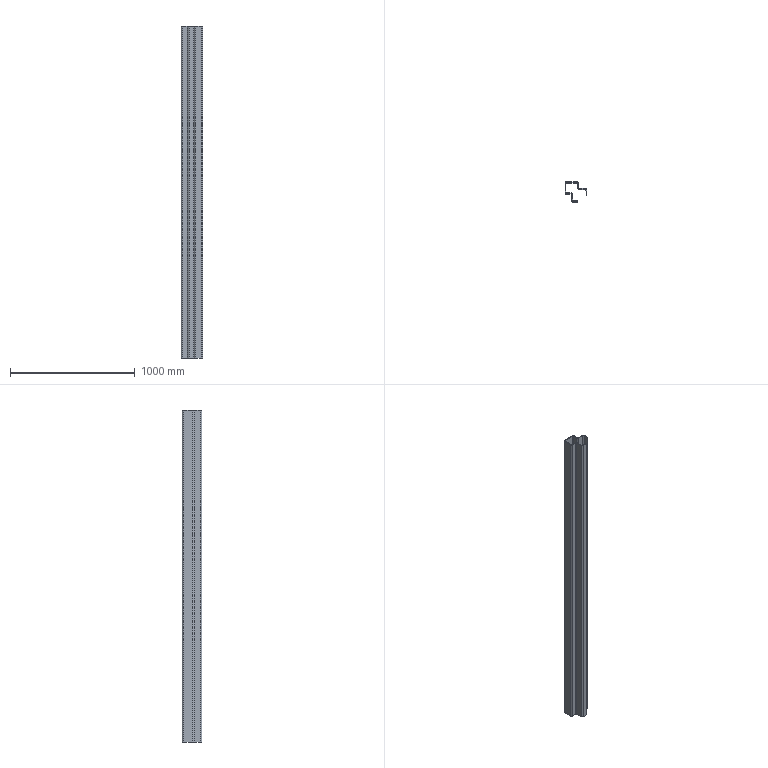Part | SolidWorks | features Extrusion 1 | 1 solid | 34 faces | box 174 x 158 x 2660 mm | volume 7867644 mm3 | plane 20 | cylinder 14 | commonest cylinder face diameters 12 x7 24 x7
STEP:
#1=CARTESIAN_POINT('',(-6.,0.,0.));
#2=VERTEX_POINT('',#1);
#3=CARTESIAN_POINT('',(0.,0.,0.));
#4=VERTEX_POINT('',#3);
#5=CARTESIAN_POINT('',(-6.,0.,0.));
#6=DIRECTION('',(1.,0.,0.));
#7=VECTOR('',#6,1000.);
#8=LINE('',#5,#7);
#9=EDGE_CURVE('',#2,#4,#8,.T.);
#10=ORIENTED_EDGE('',*,*,#9,.T.);
#11=CARTESIAN_POINT('',(0.,0.,2660.));
#12=VERTEX_POINT('',#11);
#13=CARTESIAN_POINT('',(0.,0.,2660.));
#14=DIRECTION('',(0.,0.,-1.));
#15=VECTOR('',#14,1000.);
#16=LINE('',#13,#15);
#17=EDGE_CURVE('',#12,#4,#16,.T.);
#18=ORIENTED_EDGE('',*,*,#17,.F.);
#19=CARTESIAN_POINT('',(-6.,0.,2660.));
#20=VERTEX_POINT('',#19);
#21=CARTESIAN_POINT('',(-6.,0.,2660.));
#22=DIRECTION('',(1.,0.,0.));
#23=VECTOR('',#22,1000.);
#24=LINE('',#21,#23);
#25=EDGE_CURVE('',#20,#12,#24,.T.);
#26=ORIENTED_EDGE('',*,*,#25,.F.);
#27=CARTESIAN_POINT('',(-6.,0.,2660.));
#28=DIRECTION('',(0.,0.,-1.));
#29=VECTOR('',#28,1000.);
#30=LINE('',#27,#29);
#31=EDGE_CURVE('',#20,#2,#30,.T.);
#32=ORIENTED_EDGE('',*,*,#31,.T.);
#33=EDGE_LOOP('',(#10,#18,#26,#32));
#34=FACE_OUTER_BOUND('',#33,.T.);
#35=CARTESIAN_POINT('',(-6.,0.,2660.));
#36=DIRECTION('',(0.,1.,0.));
#37=DIRECTION('',(0.,0.,1.));
#38=AXIS2_PLACEMENT_3D('',#35,#36,#37);
#39=PLANE('',#38);
#40=ADVANCED_FACE('',(#34),#39,.F.);
#41=CARTESIAN_POINT('',(0.,38.,0.));
#42=VERTEX_POINT('',#41);
#43=CARTESIAN_POINT('',(0.,0.,0.));
#44=DIRECTION('',(0.,1.,0.));
#45=VECTOR('',#44,1000.);
#46=LINE('',#43,#45);
#47=EDGE_CURVE('',#4,#42,#46,.T.);
#48=ORIENTED_EDGE('',*,*,#47,.T.);
#49=CARTESIAN_POINT('',(0.,38.,2660.));
#50=VERTEX_POINT('',#49);
#51=CARTESIAN_POINT('',(0.,38.,2660.));
#52=DIRECTION('',(0.,0.,-1.));
#53=VECTOR('',#52,1000.);
#54=LINE('',#51,#53);
#55=EDGE_CURVE('',#50,#42,#54,.T.);
#56=ORIENTED_EDGE('',*,*,#55,.F.);
#57=CARTESIAN_POINT('',(0.,0.,2660.));
#58=DIRECTION('',(0.,1.,0.));
#59=VECTOR('',#58,1000.);
#60=LINE('',#57,#59);
#61=EDGE_CURVE('',#12,#50,#60,.T.);
#62=ORIENTED_EDGE('',*,*,#61,.F.);
#63=ORIENTED_EDGE('',*,*,#17,.T.);
#64=EDGE_LOOP('',(#48,#56,#62,#63));
#65=FACE_OUTER_BOUND('',#64,.T.);
#66=CARTESIAN_POINT('',(0.,0.,2660.));
#67=DIRECTION('',(-1.,0.,0.));
#68=DIRECTION('',(0.,0.,1.));
#69=AXIS2_PLACEMENT_3D('',#66,#67,#68);
#70=PLANE('',#69);
#71=ADVANCED_FACE('',(#65),#70,.F.);
#72=CARTESIAN_POINT('',(-12.,50.,0.));
#73=VERTEX_POINT('',#72);
#74=CARTESIAN_POINT('',(-12.,38.,0.));
#75=DIRECTION('',(0.,0.,1.));
#76=DIRECTION('',(1.,0.,0.));
#77=AXIS2_PLACEMENT_3D('',#74,#75,#76);
#78=CIRCLE('',#77,12.);
#79=EDGE_CURVE('',#42,#73,#78,.T.);
#80=ORIENTED_EDGE('',*,*,#79,.T.);
#81=CARTESIAN_POINT('',(-12.,50.,2660.));
#82=VERTEX_POINT('',#81);
#83=CARTESIAN_POINT('',(-12.,50.,2660.));
#84=DIRECTION('',(0.,0.,-1.));
#85=VECTOR('',#84,1000.);
#86=LINE('',#83,#85);
#87=EDGE_CURVE('',#82,#73,#86,.T.);
#88=ORIENTED_EDGE('',*,*,#87,.F.);
#89=CARTESIAN_POINT('',(-12.,38.,2660.));
#90=DIRECTION('',(0.,0.,1.));
#91=DIRECTION('',(1.,0.,0.));
#92=AXIS2_PLACEMENT_3D('',#89,#90,#91);
#93=CIRCLE('',#92,12.);
#94=EDGE_CURVE('',#50,#82,#93,.T.);
#95=ORIENTED_EDGE('',*,*,#94,.F.);
#96=ORIENTED_EDGE('',*,*,#55,.T.);
#97=EDGE_LOOP('',(#80,#88,#95,#96));
#98=FACE_OUTER_BOUND('',#97,.T.);
#99=CARTESIAN_POINT('',(-12.,38.,2660.));
#100=DIRECTION('',(0.,0.,-1.));
#101=DIRECTION('',(-1.,0.,0.));
#102=AXIS2_PLACEMENT_3D('',#99,#100,#101);
#103=CYLINDRICAL_SURFACE('',#102,12.);
#104=ADVANCED_FACE('',(#98),#103,.T.);
#105=CARTESIAN_POINT('',(-59.,50.,0.));
#106=VERTEX_POINT('',#105);
#107=CARTESIAN_POINT('',(-12.,50.,0.));
#108=DIRECTION('',(-1.,0.,0.));
#109=VECTOR('',#108,1000.);
#110=LINE('',#107,#109);
#111=EDGE_CURVE('',#73,#106,#110,.T.);
#112=ORIENTED_EDGE('',*,*,#111,.T.);
#113=CARTESIAN_POINT('',(-59.,50.,2660.));
#114=VERTEX_POINT('',#113);
#115=CARTESIAN_POINT('',(-59.,50.,2660.));
#116=DIRECTION('',(0.,0.,-1.));
#117=VECTOR('',#116,1000.);
#118=LINE('',#115,#117);
#119=EDGE_CURVE('',#114,#106,#118,.T.);
#120=ORIENTED_EDGE('',*,*,#119,.F.);
#121=CARTESIAN_POINT('',(-12.,50.,2660.));
#122=DIRECTION('',(-1.,0.,0.));
#123=VECTOR('',#122,1000.);
#124=LINE('',#121,#123);
#125=EDGE_CURVE('',#82,#114,#124,.T.);
#126=ORIENTED_EDGE('',*,*,#125,.F.);
#127=ORIENTED_EDGE('',*,*,#87,.T.);
#128=EDGE_LOOP('',(#112,#120,#126,#127));
#129=FACE_OUTER_BOUND('',#128,.T.);
#130=CARTESIAN_POINT('',(-12.,50.,2660.));
#131=DIRECTION('',(0.,-1.,0.));
#132=DIRECTION('',(1.,0.,0.));
#133=AXIS2_PLACEMENT_3D('',#130,#131,#132);
#134=PLANE('',#133);
#135=ADVANCED_FACE('',(#129),#134,.F.);
#136=CARTESIAN_POINT('',(-65.,56.,0.));
#137=VERTEX_POINT('',#136);
#138=CARTESIAN_POINT('',(-59.,56.,0.));
#139=DIRECTION('',(0.,0.,-1.));
#140=DIRECTION('',(1.,0.,0.));
#141=AXIS2_PLACEMENT_3D('',#138,#139,#140);
#142=CIRCLE('',#141,6.);
#143=EDGE_CURVE('',#106,#137,#142,.T.);
#144=ORIENTED_EDGE('',*,*,#143,.T.);
#145=CARTESIAN_POINT('',(-65.,56.,2660.));
#146=VERTEX_POINT('',#145);
#147=CARTESIAN_POINT('',(-65.,56.,2660.));
#148=DIRECTION('',(0.,0.,-1.));
#149=VECTOR('',#148,1000.);
#150=LINE('',#147,#149);
#151=EDGE_CURVE('',#146,#137,#150,.T.);
#152=ORIENTED_EDGE('',*,*,#151,.F.);
#153=CARTESIAN_POINT('',(-59.,56.,2660.));
#154=DIRECTION('',(0.,0.,-1.));
#155=DIRECTION('',(1.,0.,0.));
#156=AXIS2_PLACEMENT_3D('',#153,#154,#155);
#157=CIRCLE('',#156,6.);
#158=EDGE_CURVE('',#114,#146,#157,.T.);
#159=ORIENTED_EDGE('',*,*,#158,.F.);
#160=ORIENTED_EDGE('',*,*,#119,.T.);
#161=EDGE_LOOP('',(#144,#152,#159,#160));
#162=FACE_OUTER_BOUND('',#161,.T.);
#163=CARTESIAN_POINT('',(-59.,56.,2660.));
#164=DIRECTION('',(0.,0.,-1.));
#165=DIRECTION('',(-1.,0.,0.));
#166=AXIS2_PLACEMENT_3D('',#163,#164,#165);
#167=CYLINDRICAL_SURFACE('',#166,6.);
#168=ADVANCED_FACE('',(#162),#167,.F.);
#169=CARTESIAN_POINT('',(-65.,91.,0.));
#170=VERTEX_POINT('',#169);
#171=CARTESIAN_POINT('',(-65.,56.,0.));
#172=DIRECTION('',(0.,1.,0.));
#173=VECTOR('',#172,1000.);
#174=LINE('',#171,#173);
#175=EDGE_CURVE('',#137,#170,#174,.T.);
#176=ORIENTED_EDGE('',*,*,#175,.T.);
#177=CARTESIAN_POINT('',(-65.,91.,2660.));
#178=VERTEX_POINT('',#177);
#179=CARTESIAN_POINT('',(-65.,91.,2660.));
#180=DIRECTION('',(0.,0.,-1.));
#181=VECTOR('',#180,1000.);
#182=LINE('',#179,#181);
#183=EDGE_CURVE('',#178,#170,#182,.T.);
#184=ORIENTED_EDGE('',*,*,#183,.F.);
#185=CARTESIAN_POINT('',(-65.,56.,2660.));
#186=DIRECTION('',(0.,1.,0.));
#187=VECTOR('',#186,1000.);
#188=LINE('',#185,#187);
#189=EDGE_CURVE('',#146,#178,#188,.T.);
#190=ORIENTED_EDGE('',*,*,#189,.F.);
#191=ORIENTED_EDGE('',*,*,#151,.T.);
#192=EDGE_LOOP('',(#176,#184,#190,#191));
#193=FACE_OUTER_BOUND('',#192,.T.);
#194=CARTESIAN_POINT('',(-65.,56.,2660.));
#195=DIRECTION('',(-1.,0.,0.));
#196=DIRECTION('',(0.,-1.,0.));
#197=AXIS2_PLACEMENT_3D('',#194,#195,#196);
#198=PLANE('',#197);
#199=ADVANCED_FACE('',(#193),#198,.F.);
#200=CARTESIAN_POINT('',(-77.,103.,0.));
#201=VERTEX_POINT('',#200);
#202=CARTESIAN_POINT('',(-77.,91.,0.));
#203=DIRECTION('',(0.,0.,1.));
#204=DIRECTION('',(1.,0.,0.));
#205=AXIS2_PLACEMENT_3D('',#202,#203,#204);
#206=CIRCLE('',#205,12.);
#207=EDGE_CURVE('',#170,#201,#206,.T.);
#208=ORIENTED_EDGE('',*,*,#207,.T.);
#209=CARTESIAN_POINT('',(-77.,103.,2660.));
#210=VERTEX_POINT('',#209);
#211=CARTESIAN_POINT('',(-77.,103.,2660.));
#212=DIRECTION('',(0.,0.,-1.));
#213=VECTOR('',#212,1000.);
#214=LINE('',#211,#213);
#215=EDGE_CURVE('',#210,#201,#214,.T.);
#216=ORIENTED_EDGE('',*,*,#215,.F.);
#217=CARTESIAN_POINT('',(-77.,91.,2660.));
#218=DIRECTION('',(0.,0.,1.));
#219=DIRECTION('',(1.,0.,0.));
#220=AXIS2_PLACEMENT_3D('',#217,#218,#219);
#221=CIRCLE('',#220,12.);
#222=EDGE_CURVE('',#178,#210,#221,.T.);
#223=ORIENTED_EDGE('',*,*,#222,.F.);
#224=ORIENTED_EDGE('',*,*,#183,.T.);
#225=EDGE_LOOP('',(#208,#216,#223,#224));
#226=FACE_OUTER_BOUND('',#225,.T.);
#227=CARTESIAN_POINT('',(-77.,91.,2660.));
#228=DIRECTION('',(0.,0.,-1.));
#229=DIRECTION('',(-1.,0.,0.));
#230=AXIS2_PLACEMENT_3D('',#227,#228,#229);
#231=CYLINDRICAL_SURFACE('',#230,12.);
#232=ADVANCED_FACE('',(#226),#231,.T.);
#233=CARTESIAN_POINT('',(-162.,103.,0.));
#234=VERTEX_POINT('',#233);
#235=CARTESIAN_POINT('',(-77.,103.,0.));
#236=DIRECTION('',(-1.,0.,0.));
#237=VECTOR('',#236,1000.);
#238=LINE('',#235,#237);
#239=EDGE_CURVE('',#201,#234,#238,.T.);
#240=ORIENTED_EDGE('',*,*,#239,.T.);
#241=CARTESIAN_POINT('',(-162.,103.,2660.));
#242=VERTEX_POINT('',#241);
#243=CARTESIAN_POINT('',(-162.,103.,2660.));
#244=DIRECTION('',(0.,0.,-1.));
#245=VECTOR('',#244,1000.);
#246=LINE('',#243,#245);
#247=EDGE_CURVE('',#242,#234,#246,.T.);
#248=ORIENTED_EDGE('',*,*,#247,.F.);
#249=CARTESIAN_POINT('',(-77.,103.,2660.));
#250=DIRECTION('',(-1.,0.,0.));
#251=VECTOR('',#250,1000.);
#252=LINE('',#249,#251);
#253=EDGE_CURVE('',#210,#242,#252,.T.);
#254=ORIENTED_EDGE('',*,*,#253,.F.);
#255=ORIENTED_EDGE('',*,*,#215,.T.);
#256=EDGE_LOOP('',(#240,#248,#254,#255));
#257=FACE_OUTER_BOUND('',#256,.T.);
#258=CARTESIAN_POINT('',(-77.,103.,2660.));
#259=DIRECTION('',(0.,-1.,0.));
#260=DIRECTION('',(1.,0.,0.));
#261=AXIS2_PLACEMENT_3D('',#258,#259,#260);
#262=PLANE('',#261);
#263=ADVANCED_FACE('',(#257),#262,.F.);
#264=CARTESIAN_POINT('',(-174.,91.,0.));
#265=VERTEX_POINT('',#264);
#266=CARTESIAN_POINT('',(-162.,91.,0.));
#267=DIRECTION('',(0.,0.,1.));
#268=DIRECTION('',(1.,0.,0.));
#269=AXIS2_PLACEMENT_3D('',#266,#267,#268);
#270=CIRCLE('',#269,12.);
#271=EDGE_CURVE('',#234,#265,#270,.T.);
#272=ORIENTED_EDGE('',*,*,#271,.T.);
#273=CARTESIAN_POINT('',(-174.,91.,2660.));
#274=VERTEX_POINT('',#273);
#275=CARTESIAN_POINT('',(-174.,91.,2660.));
#276=DIRECTION('',(0.,0.,-1.));
#277=VECTOR('',#276,1000.);
#278=LINE('',#275,#277);
#279=EDGE_CURVE('',#274,#265,#278,.T.);
#280=ORIENTED_EDGE('',*,*,#279,.F.);
#281=CARTESIAN_POINT('',(-162.,91.,2660.));
#282=DIRECTION('',(0.,0.,1.));
#283=DIRECTION('',(1.,0.,0.));
#284=AXIS2_PLACEMENT_3D('',#281,#282,#283);
#285=CIRCLE('',#284,12.);
#286=EDGE_CURVE('',#242,#274,#285,.T.);
#287=ORIENTED_EDGE('',*,*,#286,.F.);
#288=ORIENTED_EDGE('',*,*,#247,.T.);
#289=EDGE_LOOP('',(#272,#280,#287,#288));
#290=FACE_OUTER_BOUND('',#289,.T.);
#291=CARTESIAN_POINT('',(-162.,91.,2660.));
#292=DIRECTION('',(0.,0.,-1.));
#293=DIRECTION('',(-1.,0.,0.));
#294=AXIS2_PLACEMENT_3D('',#291,#292,#293);
#295=CYLINDRICAL_SURFACE('',#294,12.);
#296=ADVANCED_FACE('',(#290),#295,.T.);
#297=CARTESIAN_POINT('',(-174.,21.,0.));
#298=VERTEX_POINT('',#297);
#299=CARTESIAN_POINT('',(-174.,91.,0.));
#300=DIRECTION('',(0.,-1.,0.));
#301=VECTOR('',#300,1000.);
#302=LINE('',#299,#301);
#303=EDGE_CURVE('',#265,#298,#302,.T.);
#304=ORIENTED_EDGE('',*,*,#303,.T.);
#305=CARTESIAN_POINT('',(-174.,21.,2660.));
#306=VERTEX_POINT('',#305);
#307=CARTESIAN_POINT('',(-174.,21.,2660.));
#308=DIRECTION('',(0.,0.,-1.));
#309=VECTOR('',#308,1000.);
#310=LINE('',#307,#309);
#311=EDGE_CURVE('',#306,#298,#310,.T.);
#312=ORIENTED_EDGE('',*,*,#311,.F.);
#313=CARTESIAN_POINT('',(-174.,91.,2660.));
#314=DIRECTION('',(0.,-1.,0.));
#315=VECTOR('',#314,1000.);
#316=LINE('',#313,#315);
#317=EDGE_CURVE('',#274,#306,#316,.T.);
#318=ORIENTED_EDGE('',*,*,#317,.F.);
#319=ORIENTED_EDGE('',*,*,#279,.T.);
#320=EDGE_LOOP('',(#304,#312,#318,#319));
#321=FACE_OUTER_BOUND('',#320,.T.);
#322=CARTESIAN_POINT('',(-174.,91.,2660.));
#323=DIRECTION('',(1.,0.,0.));
#324=DIRECTION('',(0.,1.,0.));
#325=AXIS2_PLACEMENT_3D('',#322,#323,#324);
#326=PLANE('',#325);
#327=ADVANCED_FACE('',(#321),#326,.F.);
#328=CARTESIAN_POINT('',(-162.,9.,0.));
#329=VERTEX_POINT('',#328);
#330=CARTESIAN_POINT('',(-162.,21.,0.));
#331=DIRECTION('',(0.,0.,1.));
#332=DIRECTION('',(1.,0.,0.));
#333=AXIS2_PLACEMENT_3D('',#330,#331,#332);
#334=CIRCLE('',#333,12.);
#335=EDGE_CURVE('',#298,#329,#334,.T.);
#336=ORIENTED_EDGE('',*,*,#335,.T.);
#337=CARTESIAN_POINT('',(-162.,9.,2660.));
#338=VERTEX_POINT('',#337);
#339=CARTESIAN_POINT('',(-162.,9.,2660.));
#340=DIRECTION('',(0.,0.,-1.));
#341=VECTOR('',#340,1000.);
#342=LINE('',#339,#341);
#343=EDGE_CURVE('',#338,#329,#342,.T.);
#344=ORIENTED_EDGE('',*,*,#343,.F.);
#345=CARTESIAN_POINT('',(-162.,21.,2660.));
#346=DIRECTION('',(0.,0.,1.));
#347=DIRECTION('',(1.,0.,0.));
#348=AXIS2_PLACEMENT_3D('',#345,#346,#347);
#349=CIRCLE('',#348,12.);
#350=EDGE_CURVE('',#306,#338,#349,.T.);
#351=ORIENTED_EDGE('',*,*,#350,.F.);
#352=ORIENTED_EDGE('',*,*,#311,.T.);
#353=EDGE_LOOP('',(#336,#344,#351,#352));
#354=FACE_OUTER_BOUND('',#353,.T.);
#355=CARTESIAN_POINT('',(-162.,21.,2660.));
#356=DIRECTION('',(0.,0.,-1.));
#357=DIRECTION('',(-1.,0.,0.));
#358=AXIS2_PLACEMENT_3D('',#355,#356,#357);
#359=CYLINDRICAL_SURFACE('',#358,12.);
#360=ADVANCED_FACE('',(#354),#359,.T.);
#361=CARTESIAN_POINT('',(-127.,9.,0.));
#362=VERTEX_POINT('',#361);
#363=CARTESIAN_POINT('',(-162.,9.,0.));
#364=DIRECTION('',(1.,0.,0.));
#365=VECTOR('',#364,1000.);
#366=LINE('',#363,#365);
#367=EDGE_CURVE('',#329,#362,#366,.T.);
#368=ORIENTED_EDGE('',*,*,#367,.T.);
#369=CARTESIAN_POINT('',(-127.,9.,2660.));
#370=VERTEX_POINT('',#369);
#371=CARTESIAN_POINT('',(-127.,9.,2660.));
#372=DIRECTION('',(0.,0.,-1.));
#373=VECTOR('',#372,1000.);
#374=LINE('',#371,#373);
#375=EDGE_CURVE('',#370,#362,#374,.T.);
#376=ORIENTED_EDGE('',*,*,#375,.F.);
#377=CARTESIAN_POINT('',(-162.,9.,2660.));
#378=DIRECTION('',(1.,0.,0.));
#379=VECTOR('',#378,1000.);
#380=LINE('',#377,#379);
#381=EDGE_CURVE('',#338,#370,#380,.T.);
#382=ORIENTED_EDGE('',*,*,#381,.F.);
#383=ORIENTED_EDGE('',*,*,#343,.T.);
#384=EDGE_LOOP('',(#368,#376,#382,#383));
#385=FACE_OUTER_BOUND('',#384,.T.);
#386=CARTESIAN_POINT('',(-162.,9.,2660.));
#387=DIRECTION('',(0.,1.,0.));
#388=DIRECTION('',(0.,0.,1.));
#389=AXIS2_PLACEMENT_3D('',#386,#387,#388);
#390=PLANE('',#389);
#391=ADVANCED_FACE('',(#385),#390,.F.);
#392=CARTESIAN_POINT('',(-121.,3.,0.));
#393=VERTEX_POINT('',#392);
#394=CARTESIAN_POINT('',(-127.,3.,0.));
#395=DIRECTION('',(0.,0.,-1.));
#396=DIRECTION('',(1.,0.,0.));
#397=AXIS2_PLACEMENT_3D('',#394,#395,#396);
#398=CIRCLE('',#397,6.);
#399=EDGE_CURVE('',#362,#393,#398,.T.);
#400=ORIENTED_EDGE('',*,*,#399,.T.);
#401=CARTESIAN_POINT('',(-121.,3.,2660.));
#402=VERTEX_POINT('',#401);
#403=CARTESIAN_POINT('',(-121.,3.,2660.));
#404=DIRECTION('',(0.,0.,-1.));
#405=VECTOR('',#404,1000.);
#406=LINE('',#403,#405);
#407=EDGE_CURVE('',#402,#393,#406,.T.);
#408=ORIENTED_EDGE('',*,*,#407,.F.);
#409=CARTESIAN_POINT('',(-127.,3.,2660.));
#410=DIRECTION('',(0.,0.,-1.));
#411=DIRECTION('',(1.,0.,0.));
#412=AXIS2_PLACEMENT_3D('',#409,#410,#411);
#413=CIRCLE('',#412,6.);
#414=EDGE_CURVE('',#370,#402,#413,.T.);
#415=ORIENTED_EDGE('',*,*,#414,.F.);
#416=ORIENTED_EDGE('',*,*,#375,.T.);
#417=EDGE_LOOP('',(#400,#408,#415,#416));
#418=FACE_OUTER_BOUND('',#417,.T.);
#419=CARTESIAN_POINT('',(-127.,3.,2660.));
#420=DIRECTION('',(0.,0.,-1.));
#421=DIRECTION('',(-1.,0.,0.));
#422=AXIS2_PLACEMENT_3D('',#419,#420,#421);
#423=CYLINDRICAL_SURFACE('',#422,6.);
#424=ADVANCED_FACE('',(#418),#423,.F.);
#425=CARTESIAN_POINT('',(-121.,-43.,0.));
#426=VERTEX_POINT('',#425);
#427=CARTESIAN_POINT('',(-121.,3.,0.));
#428=DIRECTION('',(0.,-1.,0.));
#429=VECTOR('',#428,1000.);
#430=LINE('',#427,#429);
#431=EDGE_CURVE('',#393,#426,#430,.T.);
#432=ORIENTED_EDGE('',*,*,#431,.T.);
#433=CARTESIAN_POINT('',(-121.,-43.,2660.));
#434=VERTEX_POINT('',#433);
#435=CARTESIAN_POINT('',(-121.,-43.,2660.));
#436=DIRECTION('',(0.,0.,-1.));
#437=VECTOR('',#436,1000.);
#438=LINE('',#435,#437);
#439=EDGE_CURVE('',#434,#426,#438,.T.);
#440=ORIENTED_EDGE('',*,*,#439,.F.);
#441=CARTESIAN_POINT('',(-121.,3.,2660.));
#442=DIRECTION('',(0.,-1.,0.));
#443=VECTOR('',#442,1000.);
#444=LINE('',#441,#443);
#445=EDGE_CURVE('',#402,#434,#444,.T.);
#446=ORIENTED_EDGE('',*,*,#445,.F.);
#447=ORIENTED_EDGE('',*,*,#407,.T.);
#448=EDGE_LOOP('',(#432,#440,#446,#447));
#449=FACE_OUTER_BOUND('',#448,.T.);
#450=CARTESIAN_POINT('',(-121.,3.,2660.));
#451=DIRECTION('',(1.,0.,0.));
#452=DIRECTION('',(0.,0.,-1.));
#453=AXIS2_PLACEMENT_3D('',#450,#451,#452);
#454=PLANE('',#453);
#455=ADVANCED_FACE('',(#449),#454,.F.);
#456=CARTESIAN_POINT('',(-109.,-55.,0.));
#457=VERTEX_POINT('',#456);
#458=CARTESIAN_POINT('',(-109.,-43.,0.));
#459=DIRECTION('',(0.,0.,1.));
#460=DIRECTION('',(1.,0.,0.));
#461=AXIS2_PLACEMENT_3D('',#458,#459,#460);
#462=CIRCLE('',#461,12.);
#463=EDGE_CURVE('',#426,#457,#462,.T.);
#464=ORIENTED_EDGE('',*,*,#463,.T.);
#465=CARTESIAN_POINT('',(-109.,-55.,2660.));
#466=VERTEX_POINT('',#465);
#467=CARTESIAN_POINT('',(-109.,-55.,2660.));
#468=DIRECTION('',(0.,0.,-1.));
#469=VECTOR('',#468,1000.);
#470=LINE('',#467,#469);
#471=EDGE_CURVE('',#466,#457,#470,.T.);
#472=ORIENTED_EDGE('',*,*,#471,.F.);
#473=CARTESIAN_POINT('',(-109.,-43.,2660.));
#474=DIRECTION('',(0.,0.,1.));
#475=DIRECTION('',(1.,0.,0.));
#476=AXIS2_PLACEMENT_3D('',#473,#474,#475);
#477=CIRCLE('',#476,12.);
#478=EDGE_CURVE('',#434,#466,#477,.T.);
#479=ORIENTED_EDGE('',*,*,#478,.F.);
#480=ORIENTED_EDGE('',*,*,#439,.T.);
#481=EDGE_LOOP('',(#464,#472,#479,#480));
#482=FACE_OUTER_BOUND('',#481,.T.);
#483=CARTESIAN_POINT('',(-109.,-43.,2660.));
#484=DIRECTION('',(0.,0.,-1.));
#485=DIRECTION('',(-1.,0.,0.));
#486=AXIS2_PLACEMENT_3D('',#483,#484,#485);
#487=CYLINDRICAL_SURFACE('',#486,12.);
#488=ADVANCED_FACE('',(#482),#487,.T.);
#489=CARTESIAN_POINT('',(-71.,-55.,0.));
#490=VERTEX_POINT('',#489);
#491=CARTESIAN_POINT('',(-109.,-55.,0.));
#492=DIRECTION('',(1.,0.,0.));
#493=VECTOR('',#492,1000.);
#494=LINE('',#491,#493);
#495=EDGE_CURVE('',#457,#490,#494,.T.);
#496=ORIENTED_EDGE('',*,*,#495,.T.);
#497=CARTESIAN_POINT('',(-71.,-55.,2660.));
#498=VERTEX_POINT('',#497);
#499=CARTESIAN_POINT('',(-71.,-55.,2660.));
#500=DIRECTION('',(0.,0.,-1.));
#501=VECTOR('',#500,1000.);
#502=LINE('',#499,#501);
#503=EDGE_CURVE('',#498,#490,#502,.T.);
#504=ORIENTED_EDGE('',*,*,#503,.F.);
#505=CARTESIAN_POINT('',(-109.,-55.,2660.));
#506=DIRECTION('',(1.,0.,0.));
#507=VECTOR('',#506,1000.);
#508=LINE('',#505,#507);
#509=EDGE_CURVE('',#466,#498,#508,.T.);
#510=ORIENTED_EDGE('',*,*,#509,.F.);
#511=ORIENTED_EDGE('',*,*,#471,.T.);
#512=EDGE_LOOP('',(#496,#504,#510,#511));
#513=FACE_OUTER_BOUND('',#512,.T.);
#514=CARTESIAN_POINT('',(-109.,-55.,2660.));
#515=DIRECTION('',(0.,1.,0.));
#516=DIRECTION('',(0.,0.,1.));
#517=AXIS2_PLACEMENT_3D('',#514,#515,#516);
#518=PLANE('',#517);
#519=ADVANCED_FACE('',(#513),#518,.F.);
#520=CARTESIAN_POINT('',(-71.,-49.,0.));
#521=VERTEX_POINT('',#520);
#522=CARTESIAN_POINT('',(-71.,-55.,0.));
#523=DIRECTION('',(0.,1.,0.));
#524=VECTOR('',#523,1000.);
#525=LINE('',#522,#524);
#526=EDGE_CURVE('',#490,#521,#525,.T.);
#527=ORIENTED_EDGE('',*,*,#526,.T.);
#528=CARTESIAN_POINT('',(-71.,-49.,2660.));
#529=VERTEX_POINT('',#528);
#530=CARTESIAN_POINT('',(-71.,-49.,2660.));
#531=DIRECTION('',(0.,0.,-1.));
#532=VECTOR('',#531,1000.);
#533=LINE('',#530,#532);
#534=EDGE_CURVE('',#529,#521,#533,.T.);
#535=ORIENTED_EDGE('',*,*,#534,.F.);
#536=CARTESIAN_POINT('',(-71.,-55.,2660.));
#537=DIRECTION('',(0.,1.,0.));
#538=VECTOR('',#537,1000.);
#539=LINE('',#536,#538);
#540=EDGE_CURVE('',#498,#529,#539,.T.);
#541=ORIENTED_EDGE('',*,*,#540,.F.);
#542=ORIENTED_EDGE('',*,*,#503,.T.);
#543=EDGE_LOOP('',(#527,#535,#541,#542));
#544=FACE_OUTER_BOUND('',#543,.T.);
#545=CARTESIAN_POINT('',(-71.,-55.,2660.));
#546=DIRECTION('',(-1.,0.,0.));
#547=DIRECTION('',(0.,0.,1.));
#548=AXIS2_PLACEMENT_3D('',#545,#546,#547);
#549=PLANE('',#548);
#550=ADVANCED_FACE('',(#544),#549,.F.);
#551=CARTESIAN_POINT('',(-109.,-49.,0.));
#552=VERTEX_POINT('',#551);
#553=CARTESIAN_POINT('',(-71.,-49.,0.));
#554=DIRECTION('',(-1.,0.,0.));
#555=VECTOR('',#554,1000.);
#556=LINE('',#553,#555);
#557=EDGE_CURVE('',#521,#552,#556,.T.);
#558=ORIENTED_EDGE('',*,*,#557,.T.);
#559=CARTESIAN_POINT('',(-109.,-49.,2660.));
#560=VERTEX_POINT('',#559);
#561=CARTESIAN_POINT('',(-109.,-49.,2660.));
#562=DIRECTION('',(0.,0.,-1.));
#563=VECTOR('',#562,1000.);
#564=LINE('',#561,#563);
#565=EDGE_CURVE('',#560,#552,#564,.T.);
#566=ORIENTED_EDGE('',*,*,#565,.F.);
#567=CARTESIAN_POINT('',(-71.,-49.,2660.));
#568=DIRECTION('',(-1.,0.,0.));
#569=VECTOR('',#568,1000.);
#570=LINE('',#567,#569);
#571=EDGE_CURVE('',#529,#560,#570,.T.);
#572=ORIENTED_EDGE('',*,*,#571,.F.);
#573=ORIENTED_EDGE('',*,*,#534,.T.);
#574=EDGE_LOOP('',(#558,#566,#572,#573));
#575=FACE_OUTER_BOUND('',#574,.T.);
#576=CARTESIAN_POINT('',(-71.,-49.,2660.));
#577=DIRECTION('',(0.,-1.,0.));
#578=DIRECTION('',(0.,0.,-1.));
#579=AXIS2_PLACEMENT_3D('',#576,#577,#578);
#580=PLANE('',#579);
#581=ADVANCED_FACE('',(#575),#580,.F.);
#582=CARTESIAN_POINT('',(-115.,-43.,0.));
#583=VERTEX_POINT('',#582);
#584=CARTESIAN_POINT('',(-109.,-43.,0.));
#585=DIRECTION('',(0.,0.,-1.));
#586=DIRECTION('',(1.,0.,0.));
#587=AXIS2_PLACEMENT_3D('',#584,#585,#586);
#588=CIRCLE('',#587,6.);
#589=EDGE_CURVE('',#552,#583,#588,.T.);
#590=ORIENTED_EDGE('',*,*,#589,.T.);
#591=CARTESIAN_POINT('',(-115.,-43.,2660.));
#592=VERTEX_POINT('',#591);
#593=CARTESIAN_POINT('',(-115.,-43.,2660.));
#594=DIRECTION('',(0.,0.,-1.));
#595=VECTOR('',#594,1000.);
#596=LINE('',#593,#595);
#597=EDGE_CURVE('',#592,#583,#596,.T.);
#598=ORIENTED_EDGE('',*,*,#597,.F.);
#599=CARTESIAN_POINT('',(-109.,-43.,2660.));
#600=DIRECTION('',(0.,0.,-1.));
#601=DIRECTION('',(1.,0.,0.));
#602=AXIS2_PLACEMENT_3D('',#599,#600,#601);
#603=CIRCLE('',#602,6.);
#604=EDGE_CURVE('',#560,#592,#603,.T.);
#605=ORIENTED_EDGE('',*,*,#604,.F.);
#606=ORIENTED_EDGE('',*,*,#565,.T.);
#607=EDGE_LOOP('',(#590,#598,#605,#606));
#608=FACE_OUTER_BOUND('',#607,.T.);
#609=CARTESIAN_POINT('',(-109.,-43.,2660.));
#610=DIRECTION('',(0.,0.,-1.));
#611=DIRECTION('',(-1.,0.,0.));
#612=AXIS2_PLACEMENT_3D('',#609,#610,#611);
#613=CYLINDRICAL_SURFACE('',#612,6.);
#614=ADVANCED_FACE('',(#608),#613,.F.);
#615=CARTESIAN_POINT('',(-115.,3.,0.));
#616=VERTEX_POINT('',#615);
#617=CARTESIAN_POINT('',(-115.,-43.,0.));
#618=DIRECTION('',(0.,1.,0.));
#619=VECTOR('',#618,1000.);
#620=LINE('',#617,#619);
#621=EDGE_CURVE('',#583,#616,#620,.T.);
#622=ORIENTED_EDGE('',*,*,#621,.T.);
#623=CARTESIAN_POINT('',(-115.,3.,2660.));
#624=VERTEX_POINT('',#623);
#625=CARTESIAN_POINT('',(-115.,3.,2660.));
#626=DIRECTION('',(0.,0.,-1.));
#627=VECTOR('',#626,1000.);
#628=LINE('',#625,#627);
#629=EDGE_CURVE('',#624,#616,#628,.T.);
#630=ORIENTED_EDGE('',*,*,#629,.F.);
#631=CARTESIAN_POINT('',(-115.,-43.,2660.));
#632=DIRECTION('',(0.,1.,0.));
#633=VECTOR('',#632,1000.);
#634=LINE('',#631,#633);
#635=EDGE_CURVE('',#592,#624,#634,.T.);
#636=ORIENTED_EDGE('',*,*,#635,.F.);
#637=ORIENTED_EDGE('',*,*,#597,.T.);
#638=EDGE_LOOP('',(#622,#630,#636,#637));
#639=FACE_OUTER_BOUND('',#638,.T.);
#640=CARTESIAN_POINT('',(-115.,-43.,2660.));
#641=DIRECTION('',(-1.,0.,0.));
#642=DIRECTION('',(0.,0.,1.));
#643=AXIS2_PLACEMENT_3D('',#640,#641,#642);
#644=PLANE('',#643);
#645=ADVANCED_FACE('',(#639),#644,.F.);
#646=CARTESIAN_POINT('',(-127.,15.,0.));
#647=VERTEX_POINT('',#646);
#648=CARTESIAN_POINT('',(-127.,3.,0.));
#649=DIRECTION('',(0.,0.,1.));
#650=DIRECTION('',(1.,0.,0.));
#651=AXIS2_PLACEMENT_3D('',#648,#649,#650);
#652=CIRCLE('',#651,12.);
#653=EDGE_CURVE('',#616,#647,#652,.T.);
#654=ORIENTED_EDGE('',*,*,#653,.T.);
#655=CARTESIAN_POINT('',(-127.,15.,2660.));
#656=VERTEX_POINT('',#655);
#657=CARTESIAN_POINT('',(-127.,15.,2660.));
#658=DIRECTION('',(0.,0.,-1.));
#659=VECTOR('',#658,1000.);
#660=LINE('',#657,#659);
#661=EDGE_CURVE('',#656,#647,#660,.T.);
#662=ORIENTED_EDGE('',*,*,#661,.F.);
#663=CARTESIAN_POINT('',(-127.,3.,2660.));
#664=DIRECTION('',(0.,0.,1.));
#665=DIRECTION('',(1.,0.,0.));
#666=AXIS2_PLACEMENT_3D('',#663,#664,#665);
#667=CIRCLE('',#666,12.);
#668=EDGE_CURVE('',#624,#656,#667,.T.);
#669=ORIENTED_EDGE('',*,*,#668,.F.);
#670=ORIENTED_EDGE('',*,*,#629,.T.);
#671=EDGE_LOOP('',(#654,#662,#669,#670));
#672=FACE_OUTER_BOUND('',#671,.T.);
#673=CARTESIAN_POINT('',(-127.,3.,2660.));
#674=DIRECTION('',(0.,0.,-1.));
#675=DIRECTION('',(-1.,0.,0.));
#676=AXIS2_PLACEMENT_3D('',#673,#674,#675);
#677=CYLINDRICAL_SURFACE('',#676,12.);
#678=ADVANCED_FACE('',(#672),#677,.T.);
#679=CARTESIAN_POINT('',(-162.,15.,0.));
#680=VERTEX_POINT('',#679);
#681=CARTESIAN_POINT('',(-127.,15.,0.));
#682=DIRECTION('',(-1.,0.,0.));
#683=VECTOR('',#682,1000.);
#684=LINE('',#681,#683);
#685=EDGE_CURVE('',#647,#680,#684,.T.);
#686=ORIENTED_EDGE('',*,*,#685,.T.);
#687=CARTESIAN_POINT('',(-162.,15.,2660.));
#688=VERTEX_POINT('',#687);
#689=CARTESIAN_POINT('',(-162.,15.,2660.));
#690=DIRECTION('',(0.,0.,-1.));
#691=VECTOR('',#690,1000.);
#692=LINE('',#689,#691);
#693=EDGE_CURVE('',#688,#680,#692,.T.);
#694=ORIENTED_EDGE('',*,*,#693,.F.);
#695=CARTESIAN_POINT('',(-127.,15.,2660.));
#696=DIRECTION('',(-1.,0.,0.));
#697=VECTOR('',#696,1000.);
#698=LINE('',#695,#697);
#699=EDGE_CURVE('',#656,#688,#698,.T.);
#700=ORIENTED_EDGE('',*,*,#699,.F.);
#701=ORIENTED_EDGE('',*,*,#661,.T.);
#702=EDGE_LOOP('',(#686,#694,#700,#701));
#703=FACE_OUTER_BOUND('',#702,.T.);
#704=CARTESIAN_POINT('',(-127.,15.,2660.));
#705=DIRECTION('',(0.,-1.,0.));
#706=DIRECTION('',(0.,0.,-1.));
#707=AXIS2_PLACEMENT_3D('',#704,#705,#706);
#708=PLANE('',#707);
#709=ADVANCED_FACE('',(#703),#708,.F.);
#710=CARTESIAN_POINT('',(-168.,21.,0.));
#711=VERTEX_POINT('',#710);
#712=CARTESIAN_POINT('',(-162.,21.,0.));
#713=DIRECTION('',(0.,0.,-1.));
#714=DIRECTION('',(1.,0.,0.));
#715=AXIS2_PLACEMENT_3D('',#712,#713,#714);
#716=CIRCLE('',#715,6.);
#717=EDGE_CURVE('',#680,#711,#716,.T.);
#718=ORIENTED_EDGE('',*,*,#717,.T.);
#719=CARTESIAN_POINT('',(-168.,21.,2660.));
#720=VERTEX_POINT('',#719);
#721=CARTESIAN_POINT('',(-168.,21.,2660.));
#722=DIRECTION('',(0.,0.,-1.));
#723=VECTOR('',#722,1000.);
#724=LINE('',#721,#723);
#725=EDGE_CURVE('',#720,#711,#724,.T.);
#726=ORIENTED_EDGE('',*,*,#725,.F.);
#727=CARTESIAN_POINT('',(-162.,21.,2660.));
#728=DIRECTION('',(0.,0.,-1.));
#729=DIRECTION('',(1.,0.,0.));
#730=AXIS2_PLACEMENT_3D('',#727,#728,#729);
#731=CIRCLE('',#730,6.);
#732=EDGE_CURVE('',#688,#720,#731,.T.);
#733=ORIENTED_EDGE('',*,*,#732,.F.);
#734=ORIENTED_EDGE('',*,*,#693,.T.);
#735=EDGE_LOOP('',(#718,#726,#733,#734));
#736=FACE_OUTER_BOUND('',#735,.T.);
#737=CARTESIAN_POINT('',(-162.,21.,2660.));
#738=DIRECTION('',(0.,0.,-1.));
#739=DIRECTION('',(-1.,0.,0.));
#740=AXIS2_PLACEMENT_3D('',#737,#738,#739);
#741=CYLINDRICAL_SURFACE('',#740,6.);
#742=ADVANCED_FACE('',(#736),#741,.F.);
#743=CARTESIAN_POINT('',(-168.,91.,0.));
#744=VERTEX_POINT('',#743);
#745=CARTESIAN_POINT('',(-168.,21.,0.));
#746=DIRECTION('',(0.,1.,0.));
#747=VECTOR('',#746,1000.);
#748=LINE('',#745,#747);
#749=EDGE_CURVE('',#711,#744,#748,.T.);
#750=ORIENTED_EDGE('',*,*,#749,.T.);
#751=CARTESIAN_POINT('',(-168.,91.,2660.));
#752=VERTEX_POINT('',#751);
#753=CARTESIAN_POINT('',(-168.,91.,2660.));
#754=DIRECTION('',(0.,0.,-1.));
#755=VECTOR('',#754,1000.);
#756=LINE('',#753,#755);
#757=EDGE_CURVE('',#752,#744,#756,.T.);
#758=ORIENTED_EDGE('',*,*,#757,.F.);
#759=CARTESIAN_POINT('',(-168.,21.,2660.));
#760=DIRECTION('',(0.,1.,0.));
#761=VECTOR('',#760,1000.);
#762=LINE('',#759,#761);
#763=EDGE_CURVE('',#720,#752,#762,.T.);
#764=ORIENTED_EDGE('',*,*,#763,.F.);
#765=ORIENTED_EDGE('',*,*,#725,.T.);
#766=EDGE_LOOP('',(#750,#758,#764,#765));
#767=FACE_OUTER_BOUND('',#766,.T.);
#768=CARTESIAN_POINT('',(-168.,21.,2660.));
#769=DIRECTION('',(-1.,0.,0.));
#770=DIRECTION('',(0.,-1.,0.));
#771=AXIS2_PLACEMENT_3D('',#768,#769,#770);
#772=PLANE('',#771);
#773=ADVANCED_FACE('',(#767),#772,.F.);
#774=CARTESIAN_POINT('',(-162.,97.,0.));
#775=VERTEX_POINT('',#774);
#776=CARTESIAN_POINT('',(-162.,91.,0.));
#777=DIRECTION('',(0.,0.,-1.));
#778=DIRECTION('',(1.,0.,0.));
#779=AXIS2_PLACEMENT_3D('',#776,#777,#778);
#780=CIRCLE('',#779,6.);
#781=EDGE_CURVE('',#744,#775,#780,.T.);
#782=ORIENTED_EDGE('',*,*,#781,.T.);
#783=CARTESIAN_POINT('',(-162.,97.,2660.));
#784=VERTEX_POINT('',#783);
#785=CARTESIAN_POINT('',(-162.,97.,2660.));
#786=DIRECTION('',(0.,0.,-1.));
#787=VECTOR('',#786,1000.);
#788=LINE('',#785,#787);
#789=EDGE_CURVE('',#784,#775,#788,.T.);
#790=ORIENTED_EDGE('',*,*,#789,.F.);
#791=CARTESIAN_POINT('',(-162.,91.,2660.));
#792=DIRECTION('',(0.,0.,-1.));
#793=DIRECTION('',(1.,0.,0.));
#794=AXIS2_PLACEMENT_3D('',#791,#792,#793);
#795=CIRCLE('',#794,6.);
#796=EDGE_CURVE('',#752,#784,#795,.T.);
#797=ORIENTED_EDGE('',*,*,#796,.F.);
#798=ORIENTED_EDGE('',*,*,#757,.T.);
#799=EDGE_LOOP('',(#782,#790,#797,#798));
#800=FACE_OUTER_BOUND('',#799,.T.);
#801=CARTESIAN_POINT('',(-162.,91.,2660.));
#802=DIRECTION('',(0.,0.,-1.));
#803=DIRECTION('',(-1.,0.,0.));
#804=AXIS2_PLACEMENT_3D('',#801,#802,#803);
#805=CYLINDRICAL_SURFACE('',#804,6.);
#806=ADVANCED_FACE('',(#800),#805,.F.);
#807=CARTESIAN_POINT('',(-77.,97.,0.));
#808=VERTEX_POINT('',#807);
#809=CARTESIAN_POINT('',(-162.,97.,0.));
#810=DIRECTION('',(1.,0.,0.));
#811=VECTOR('',#810,1000.);
#812=LINE('',#809,#811);
#813=EDGE_CURVE('',#775,#808,#812,.T.);
#814=ORIENTED_EDGE('',*,*,#813,.T.);
#815=CARTESIAN_POINT('',(-77.,97.,2660.));
#816=VERTEX_POINT('',#815);
#817=CARTESIAN_POINT('',(-77.,97.,2660.));
#818=DIRECTION('',(0.,0.,-1.));
#819=VECTOR('',#818,1000.);
#820=LINE('',#817,#819);
#821=EDGE_CURVE('',#816,#808,#820,.T.);
#822=ORIENTED_EDGE('',*,*,#821,.F.);
#823=CARTESIAN_POINT('',(-162.,97.,2660.));
#824=DIRECTION('',(1.,0.,0.));
#825=VECTOR('',#824,1000.);
#826=LINE('',#823,#825);
#827=EDGE_CURVE('',#784,#816,#826,.T.);
#828=ORIENTED_EDGE('',*,*,#827,.F.);
#829=ORIENTED_EDGE('',*,*,#789,.T.);
#830=EDGE_LOOP('',(#814,#822,#828,#829));
#831=FACE_OUTER_BOUND('',#830,.T.);
#832=CARTESIAN_POINT('',(-162.,97.,2660.));
#833=DIRECTION('',(0.,1.,0.));
#834=DIRECTION('',(-1.,0.,0.));
#835=AXIS2_PLACEMENT_3D('',#832,#833,#834);
#836=PLANE('',#835);
#837=ADVANCED_FACE('',(#831),#836,.F.);
#838=CARTESIAN_POINT('',(-71.,91.,0.));
#839=VERTEX_POINT('',#838);
#840=CARTESIAN_POINT('',(-77.,91.,0.));
#841=DIRECTION('',(0.,0.,-1.));
#842=DIRECTION('',(1.,0.,0.));
#843=AXIS2_PLACEMENT_3D('',#840,#841,#842);
#844=CIRCLE('',#843,6.);
#845=EDGE_CURVE('',#808,#839,#844,.T.);
#846=ORIENTED_EDGE('',*,*,#845,.T.);
#847=CARTESIAN_POINT('',(-71.,91.,2660.));
#848=VERTEX_POINT('',#847);
#849=CARTESIAN_POINT('',(-71.,91.,2660.));
#850=DIRECTION('',(0.,0.,-1.));
#851=VECTOR('',#850,1000.);
#852=LINE('',#849,#851);
#853=EDGE_CURVE('',#848,#839,#852,.T.);
#854=ORIENTED_EDGE('',*,*,#853,.F.);
#855=CARTESIAN_POINT('',(-77.,91.,2660.));
#856=DIRECTION('',(0.,0.,-1.));
#857=DIRECTION('',(1.,0.,0.));
#858=AXIS2_PLACEMENT_3D('',#855,#856,#857);
#859=CIRCLE('',#858,6.);
#860=EDGE_CURVE('',#816,#848,#859,.T.);
#861=ORIENTED_EDGE('',*,*,#860,.F.);
#862=ORIENTED_EDGE('',*,*,#821,.T.);
#863=EDGE_LOOP('',(#846,#854,#861,#862));
#864=FACE_OUTER_BOUND('',#863,.T.);
#865=CARTESIAN_POINT('',(-77.,91.,2660.));
#866=DIRECTION('',(0.,0.,-1.));
#867=DIRECTION('',(-1.,0.,0.));
#868=AXIS2_PLACEMENT_3D('',#865,#866,#867);
#869=CYLINDRICAL_SURFACE('',#868,6.);
#870=ADVANCED_FACE('',(#864),#869,.F.);
#871=CARTESIAN_POINT('',(-71.,56.,0.));
#872=VERTEX_POINT('',#871);
#873=CARTESIAN_POINT('',(-71.,91.,0.));
#874=DIRECTION('',(0.,-1.,0.));
#875=VECTOR('',#874,1000.);
#876=LINE('',#873,#875);
#877=EDGE_CURVE('',#839,#872,#876,.T.);
#878=ORIENTED_EDGE('',*,*,#877,.T.);
#879=CARTESIAN_POINT('',(-71.,56.,2660.));
#880=VERTEX_POINT('',#879);
#881=CARTESIAN_POINT('',(-71.,56.,2660.));
#882=DIRECTION('',(0.,0.,-1.));
#883=VECTOR('',#882,1000.);
#884=LINE('',#881,#883);
#885=EDGE_CURVE('',#880,#872,#884,.T.);
#886=ORIENTED_EDGE('',*,*,#885,.F.);
#887=CARTESIAN_POINT('',(-71.,91.,2660.));
#888=DIRECTION('',(0.,-1.,0.));
#889=VECTOR('',#888,1000.);
#890=LINE('',#887,#889);
#891=EDGE_CURVE('',#848,#880,#890,.T.);
#892=ORIENTED_EDGE('',*,*,#891,.F.);
#893=ORIENTED_EDGE('',*,*,#853,.T.);
#894=EDGE_LOOP('',(#878,#886,#892,#893));
#895=FACE_OUTER_BOUND('',#894,.T.);
#896=CARTESIAN_POINT('',(-71.,91.,2660.));
#897=DIRECTION('',(1.,0.,0.));
#898=DIRECTION('',(0.,1.,0.));
#899=AXIS2_PLACEMENT_3D('',#896,#897,#898);
#900=PLANE('',#899);
#901=ADVANCED_FACE('',(#895),#900,.F.);
#902=CARTESIAN_POINT('',(-59.,44.,0.));
#903=VERTEX_POINT('',#902);
#904=CARTESIAN_POINT('',(-59.,56.,0.));
#905=DIRECTION('',(0.,0.,1.));
#906=DIRECTION('',(1.,0.,0.));
#907=AXIS2_PLACEMENT_3D('',#904,#905,#906);
#908=CIRCLE('',#907,12.);
#909=EDGE_CURVE('',#872,#903,#908,.T.);
#910=ORIENTED_EDGE('',*,*,#909,.T.);
#911=CARTESIAN_POINT('',(-59.,44.,2660.));
#912=VERTEX_POINT('',#911);
#913=CARTESIAN_POINT('',(-59.,44.,2660.));
#914=DIRECTION('',(0.,0.,-1.));
#915=VECTOR('',#914,1000.);
#916=LINE('',#913,#915);
#917=EDGE_CURVE('',#912,#903,#916,.T.);
#918=ORIENTED_EDGE('',*,*,#917,.F.);
#919=CARTESIAN_POINT('',(-59.,56.,2660.));
#920=DIRECTION('',(0.,0.,1.));
#921=DIRECTION('',(1.,0.,0.));
#922=AXIS2_PLACEMENT_3D('',#919,#920,#921);
#923=CIRCLE('',#922,12.);
#924=EDGE_CURVE('',#880,#912,#923,.T.);
#925=ORIENTED_EDGE('',*,*,#924,.F.);
#926=ORIENTED_EDGE('',*,*,#885,.T.);
#927=EDGE_LOOP('',(#910,#918,#925,#926));
#928=FACE_OUTER_BOUND('',#927,.T.);
#929=CARTESIAN_POINT('',(-59.,56.,2660.));
#930=DIRECTION('',(0.,0.,-1.));
#931=DIRECTION('',(-1.,0.,0.));
#932=AXIS2_PLACEMENT_3D('',#929,#930,#931);
#933=CYLINDRICAL_SURFACE('',#932,12.);
#934=ADVANCED_FACE('',(#928),#933,.T.);
#935=CARTESIAN_POINT('',(-12.,44.,0.));
#936=VERTEX_POINT('',#935);
#937=CARTESIAN_POINT('',(-59.,44.,0.));
#938=DIRECTION('',(1.,0.,0.));
#939=VECTOR('',#938,1000.);
#940=LINE('',#937,#939);
#941=EDGE_CURVE('',#903,#936,#940,.T.);
#942=ORIENTED_EDGE('',*,*,#941,.T.);
#943=CARTESIAN_POINT('',(-12.,44.,2660.));
#944=VERTEX_POINT('',#943);
#945=CARTESIAN_POINT('',(-12.,44.,2660.));
#946=DIRECTION('',(0.,0.,-1.));
#947=VECTOR('',#946,1000.);
#948=LINE('',#945,#947);
#949=EDGE_CURVE('',#944,#936,#948,.T.);
#950=ORIENTED_EDGE('',*,*,#949,.F.);
#951=CARTESIAN_POINT('',(-59.,44.,2660.));
#952=DIRECTION('',(1.,0.,0.));
#953=VECTOR('',#952,1000.);
#954=LINE('',#951,#953);
#955=EDGE_CURVE('',#912,#944,#954,.T.);
#956=ORIENTED_EDGE('',*,*,#955,.F.);
#957=ORIENTED_EDGE('',*,*,#917,.T.);
#958=EDGE_LOOP('',(#942,#950,#956,#957));
#959=FACE_OUTER_BOUND('',#958,.T.);
#960=CARTESIAN_POINT('',(-59.,44.,2660.));
#961=DIRECTION('',(0.,1.,0.));
#962=DIRECTION('',(-1.,0.,0.));
#963=AXIS2_PLACEMENT_3D('',#960,#961,#962);
#964=PLANE('',#963);
#965=ADVANCED_FACE('',(#959),#964,.F.);
#966=CARTESIAN_POINT('',(-6.,38.,0.));
#967=VERTEX_POINT('',#966);
#968=CARTESIAN_POINT('',(-12.,38.,0.));
#969=DIRECTION('',(0.,0.,-1.));
#970=DIRECTION('',(1.,0.,0.));
#971=AXIS2_PLACEMENT_3D('',#968,#969,#970);
#972=CIRCLE('',#971,6.);
#973=EDGE_CURVE('',#936,#967,#972,.T.);
#974=ORIENTED_EDGE('',*,*,#973,.T.);
#975=CARTESIAN_POINT('',(-6.,38.,2660.));
#976=VERTEX_POINT('',#975);
#977=CARTESIAN_POINT('',(-6.,38.,2660.));
#978=DIRECTION('',(0.,0.,-1.));
#979=VECTOR('',#978,1000.);
#980=LINE('',#977,#979);
#981=EDGE_CURVE('',#976,#967,#980,.T.);
#982=ORIENTED_EDGE('',*,*,#981,.F.);
#983=CARTESIAN_POINT('',(-12.,38.,2660.));
#984=DIRECTION('',(0.,0.,-1.));
#985=DIRECTION('',(1.,0.,0.));
#986=AXIS2_PLACEMENT_3D('',#983,#984,#985);
#987=CIRCLE('',#986,6.);
#988=EDGE_CURVE('',#944,#976,#987,.T.);
#989=ORIENTED_EDGE('',*,*,#988,.F.);
#990=ORIENTED_EDGE('',*,*,#949,.T.);
#991=EDGE_LOOP('',(#974,#982,#989,#990));
#992=FACE_OUTER_BOUND('',#991,.T.);
#993=CARTESIAN_POINT('',(-12.,38.,2660.));
#994=DIRECTION('',(0.,0.,-1.));
#995=DIRECTION('',(-1.,0.,0.));
#996=AXIS2_PLACEMENT_3D('',#993,#994,#995);
#997=CYLINDRICAL_SURFACE('',#996,6.);
#998=ADVANCED_FACE('',(#992),#997,.F.);
#999=CARTESIAN_POINT('',(-6.,38.,0.));
#1000=DIRECTION('',(0.,-1.,0.));
#1001=VECTOR('',#1000,1000.);
#1002=LINE('',#999,#1001);
#1003=EDGE_CURVE('',#967,#2,#1002,.T.);
#1004=ORIENTED_EDGE('',*,*,#1003,.T.);
#1005=ORIENTED_EDGE('',*,*,#31,.F.);
#1006=CARTESIAN_POINT('',(-6.,38.,2660.));
#1007=DIRECTION('',(0.,-1.,0.));
#1008=VECTOR('',#1007,1000.);
#1009=LINE('',#1006,#1008);
#1010=EDGE_CURVE('',#976,#20,#1009,.T.);
#1011=ORIENTED_EDGE('',*,*,#1010,.F.);
#1012=ORIENTED_EDGE('',*,*,#981,.T.);
#1013=EDGE_LOOP('',(#1004,#1005,#1011,#1012));
#1014=FACE_OUTER_BOUND('',#1013,.T.);
#1015=CARTESIAN_POINT('',(-6.,38.,2660.));
#1016=DIRECTION('',(1.,0.,0.));
#1017=DIRECTION('',(0.,1.,0.));
#1018=AXIS2_PLACEMENT_3D('',#1015,#1016,#1017);
#1019=PLANE('',#1018);
#1020=ADVANCED_FACE('',(#1014),#1019,.F.);
#1021=ORIENTED_EDGE('',*,*,#25,.T.);
#1022=ORIENTED_EDGE('',*,*,#61,.T.);
#1023=ORIENTED_EDGE('',*,*,#94,.T.);
#1024=ORIENTED_EDGE('',*,*,#125,.T.);
#1025=ORIENTED_EDGE('',*,*,#158,.T.);
#1026=ORIENTED_EDGE('',*,*,#189,.T.);
#1027=ORIENTED_EDGE('',*,*,#222,.T.);
#1028=ORIENTED_EDGE('',*,*,#253,.T.);
#1029=ORIENTED_EDGE('',*,*,#286,.T.);
#1030=ORIENTED_EDGE('',*,*,#317,.T.);
#1031=ORIENTED_EDGE('',*,*,#350,.T.);
#1032=ORIENTED_EDGE('',*,*,#381,.T.);
#1033=ORIENTED_EDGE('',*,*,#414,.T.);
#1034=ORIENTED_EDGE('',*,*,#445,.T.);
#1035=ORIENTED_EDGE('',*,*,#478,.T.);
#1036=ORIENTED_EDGE('',*,*,#509,.T.);
#1037=ORIENTED_EDGE('',*,*,#540,.T.);
#1038=ORIENTED_EDGE('',*,*,#571,.T.);
#1039=ORIENTED_EDGE('',*,*,#604,.T.);
#1040=ORIENTED_EDGE('',*,*,#635,.T.);
#1041=ORIENTED_EDGE('',*,*,#668,.T.);
#1042=ORIENTED_EDGE('',*,*,#699,.T.);
#1043=ORIENTED_EDGE('',*,*,#732,.T.);
#1044=ORIENTED_EDGE('',*,*,#763,.T.);
#1045=ORIENTED_EDGE('',*,*,#796,.T.);
#1046=ORIENTED_EDGE('',*,*,#827,.T.);
#1047=ORIENTED_EDGE('',*,*,#860,.T.);
#1048=ORIENTED_EDGE('',*,*,#891,.T.);
#1049=ORIENTED_EDGE('',*,*,#924,.T.);
#1050=ORIENTED_EDGE('',*,*,#955,.T.);
#1051=ORIENTED_EDGE('',*,*,#988,.T.);
#1052=ORIENTED_EDGE('',*,*,#1010,.T.);
#1053=EDGE_LOOP('',(#1021,#1022,#1023,#1024,#1025,#1026,#1027,#1028,#1029,#1030,#1031,#1032,#1033,#1034,#1035,#1036,#1037,#1038,#1039,#1040,#1041,#1042,#1043,#1044,#1045,#1046,#1047,#1048,#1049,#1050,#1051,#1052));
#1054=FACE_OUTER_BOUND('',#1053,.T.);
#1055=CARTESIAN_POINT('',(-12.,38.,2660.));
#1056=DIRECTION('',(0.,0.,1.));
#1057=DIRECTION('',(1.,0.,0.));
#1058=AXIS2_PLACEMENT_3D('',#1055,#1056,#1057);
#1059=PLANE('',#1058);
#1060=ADVANCED_FACE('',(#1054),#1059,.T.);
#1061=ORIENTED_EDGE('',*,*,#9,.F.);
#1062=ORIENTED_EDGE('',*,*,#1003,.F.);
#1063=ORIENTED_EDGE('',*,*,#973,.F.);
#1064=ORIENTED_EDGE('',*,*,#941,.F.);
#1065=ORIENTED_EDGE('',*,*,#909,.F.);
#1066=ORIENTED_EDGE('',*,*,#877,.F.);
#1067=ORIENTED_EDGE('',*,*,#845,.F.);
#1068=ORIENTED_EDGE('',*,*,#813,.F.);
#1069=ORIENTED_EDGE('',*,*,#781,.F.);
#1070=ORIENTED_EDGE('',*,*,#749,.F.);
#1071=ORIENTED_EDGE('',*,*,#717,.F.);
#1072=ORIENTED_EDGE('',*,*,#685,.F.);
#1073=ORIENTED_EDGE('',*,*,#653,.F.);
#1074=ORIENTED_EDGE('',*,*,#621,.F.);
#1075=ORIENTED_EDGE('',*,*,#589,.F.);
#1076=ORIENTED_EDGE('',*,*,#557,.F.);
#1077=ORIENTED_EDGE('',*,*,#526,.F.);
#1078=ORIENTED_EDGE('',*,*,#495,.F.);
#1079=ORIENTED_EDGE('',*,*,#463,.F.);
#1080=ORIENTED_EDGE('',*,*,#431,.F.);
#1081=ORIENTED_EDGE('',*,*,#399,.F.);
#1082=ORIENTED_EDGE('',*,*,#367,.F.);
#1083=ORIENTED_EDGE('',*,*,#335,.F.);
#1084=ORIENTED_EDGE('',*,*,#303,.F.);
#1085=ORIENTED_EDGE('',*,*,#271,.F.);
#1086=ORIENTED_EDGE('',*,*,#239,.F.);
#1087=ORIENTED_EDGE('',*,*,#207,.F.);
#1088=ORIENTED_EDGE('',*,*,#175,.F.);
#1089=ORIENTED_EDGE('',*,*,#143,.F.);
#1090=ORIENTED_EDGE('',*,*,#111,.F.);
#1091=ORIENTED_EDGE('',*,*,#79,.F.);
#1092=ORIENTED_EDGE('',*,*,#47,.F.);
#1093=EDGE_LOOP('',(#1061,#1062,#1063,#1064,#1065,#1066,#1067,#1068,#1069,#1070,#1071,#1072,#1073,#1074,#1075,#1076,#1077,#1078,#1079,#1080,#1081,#1082,#1083,#1084,#1085,#1086,#1087,#1088,#1089,#1090,#1091,#1092));
#1094=FACE_OUTER_BOUND('',#1093,.T.);
#1095=CARTESIAN_POINT('',(-12.,38.,0.));
#1096=DIRECTION('',(0.,0.,1.));
#1097=DIRECTION('',(1.,0.,0.));
#1098=AXIS2_PLACEMENT_3D('',#1095,#1096,#1097);
#1099=PLANE('',#1098);
#1100=ADVANCED_FACE('',(#1094),#1099,.F.);
#1101=CLOSED_SHELL('',(#40,#71,#104,#135,#168,#199,#232,#263,#296,#327,#360,#391,#424,#455,#488,#519,#550,#581,#614,#645,#678,#709,#742,#773,#806,#837,#870,#901,#934,#965,#998,#1020,#1060,#1100));
#1102=MANIFOLD_SOLID_BREP('',#1101);
#1103=CARTESIAN_POINT('',(0.,0.,0.));
#1104=DIRECTION('',(0.,0.,1.));
#1105=DIRECTION('',(1.,0.,0.));
#1106=AXIS2_PLACEMENT_3D('',#1103,#1104,#1105);
#1107=(LENGTH_UNIT()NAMED_UNIT(*)SI_UNIT(.MILLI.,.METRE.));
#1108=UNCERTAINTY_MEASURE_WITH_UNIT(LENGTH_MEASURE(0.00001),#1107,'','');
#1109=(NAMED_UNIT(*)PLANE_ANGLE_UNIT()SI_UNIT($,.RADIAN.));
#1110=(NAMED_UNIT(*)SI_UNIT($,.STERADIAN.)SOLID_ANGLE_UNIT());
#1111=(GEOMETRIC_REPRESENTATION_CONTEXT(3)GLOBAL_UNCERTAINTY_ASSIGNED_CONTEXT((#1108))GLOBAL_UNIT_ASSIGNED_CONTEXT((#1107,#1109,#1110))REPRESENTATION_CONTEXT('',''));
#1112=ADVANCED_BREP_SHAPE_REPRESENTATION('',(#1102,#1106),#1111);